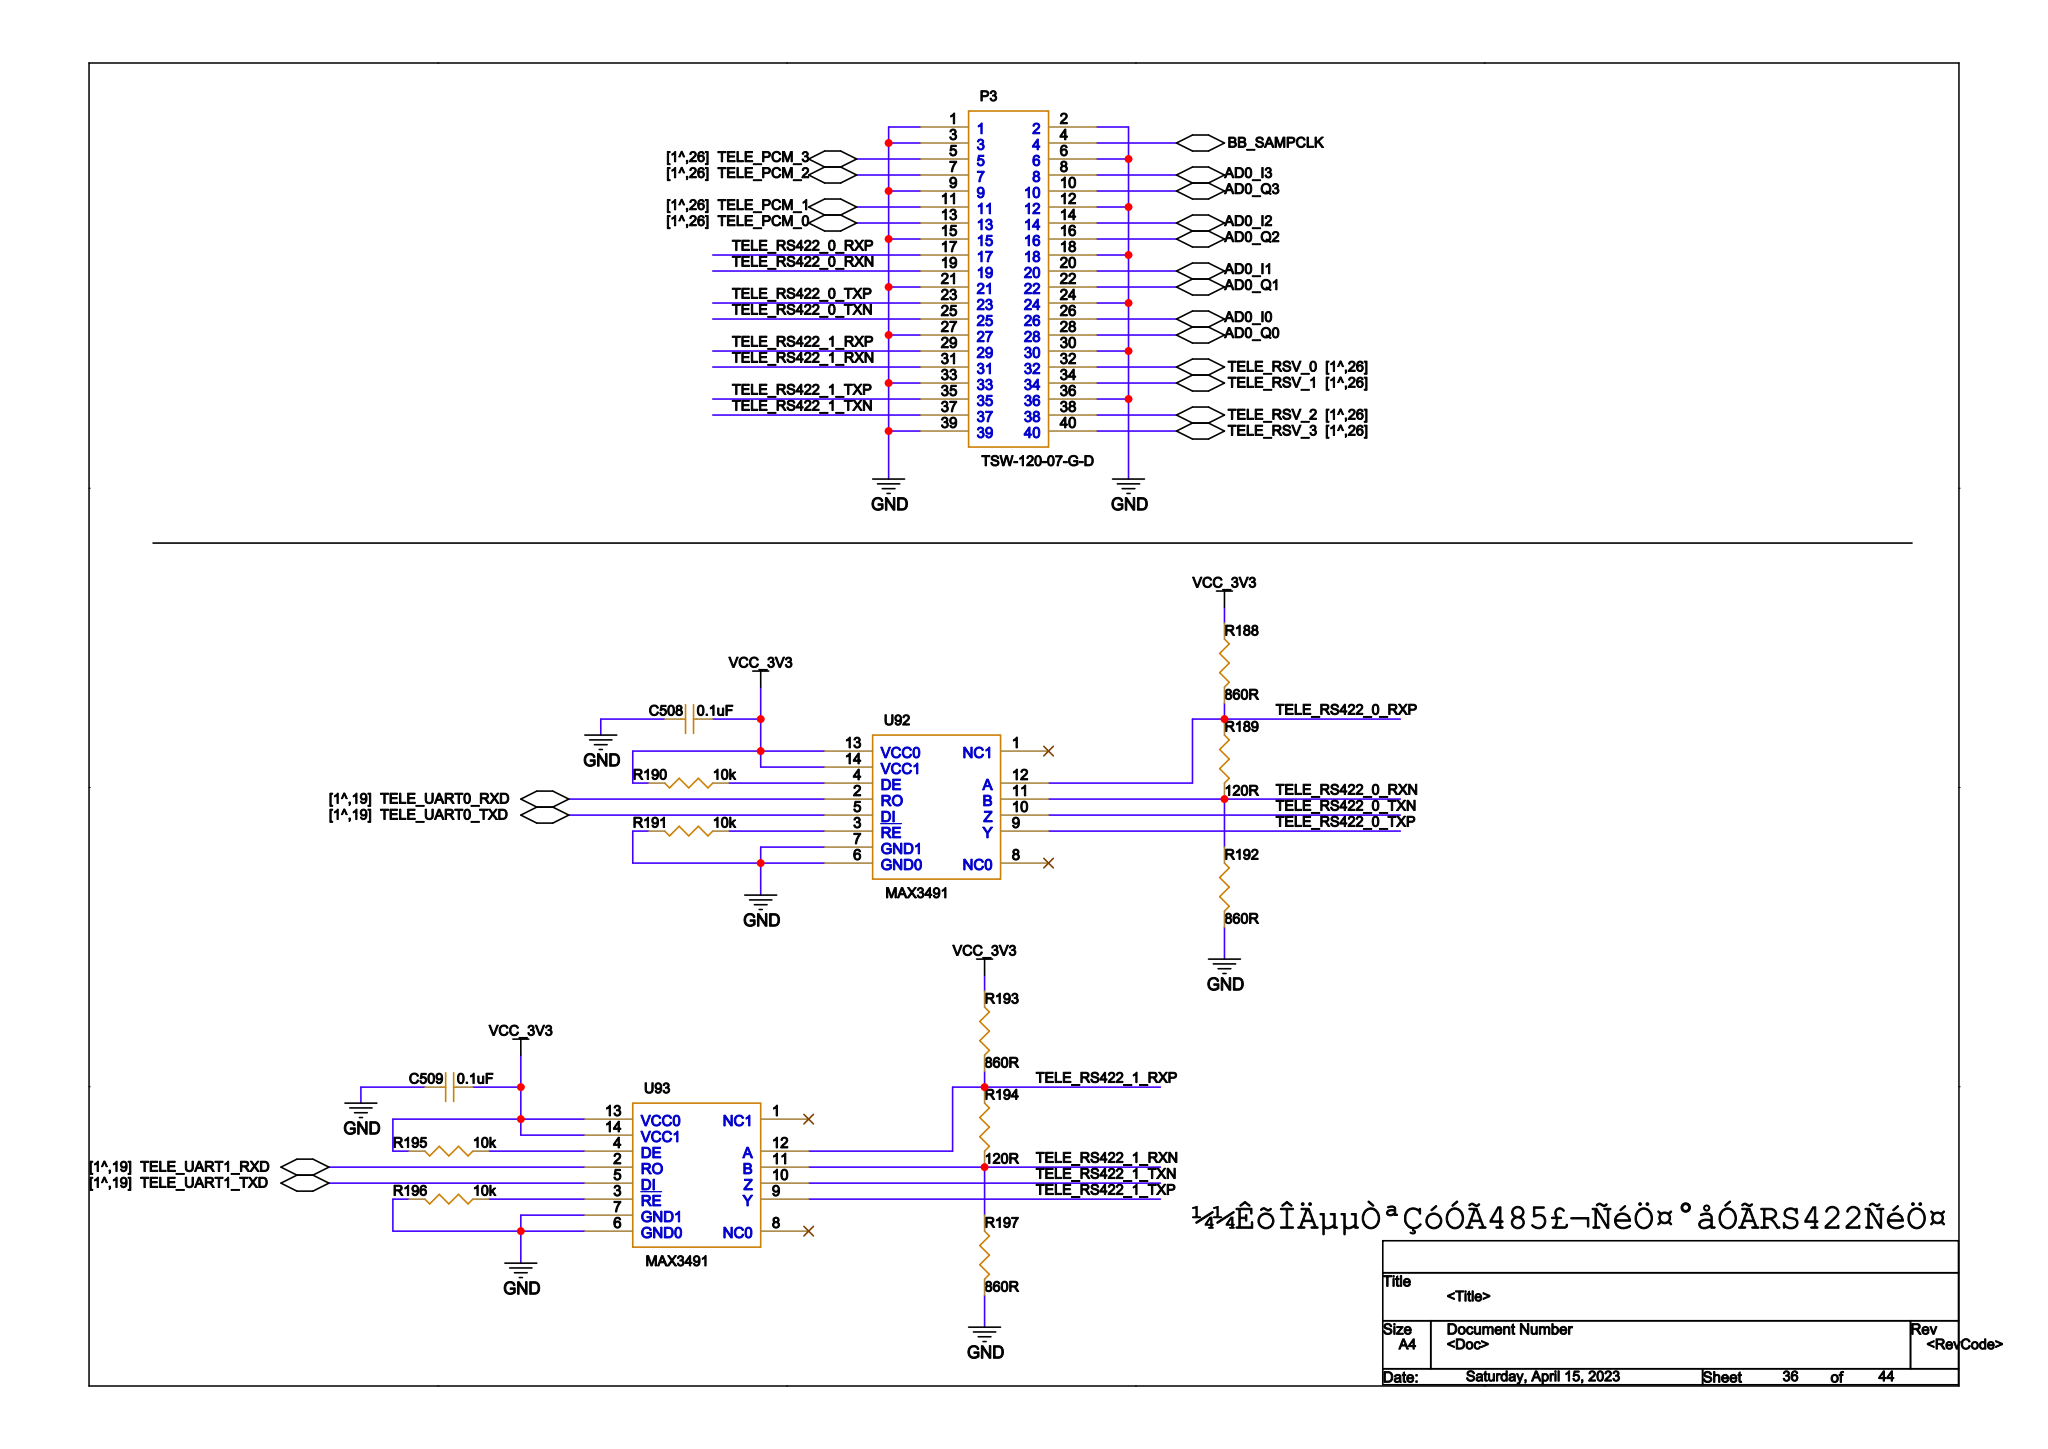Circuit board | Cadence Allegro | 1034 parts | 912 nets | one sheet of the schematic
Parts on this sheet (reference | value | footprint):
C508 | 0.1uF | C0402
C509 | 0.1uF | C0402
P3 | TSW-120-07-G-D | TSW_2MM54_DR
R188 | 860R | R0402
R189 | 120R | R0402
R190 | 10k | R0402
R191 | 10k | R0402
R192 | 860R | R0402
R193 | 860R | R0402
R194 | 120R | R0402
R195 | 10k | R0402
R196 | 10k | R0402
R197 | 860R | R0402
U92 | MAX3491 | MAX3491_14SO
U93 | MAX3491 | MAX3491_14SO
Nets of these parts (net: part-pin ...):
GND: C508-2 C509-2 R191-2 R192-2 R196-2 R197-2 U92-6 U92-7 U93-6 U93-7 P3-1 P3-2 P3-3 P3-6 P3-9 P3-12 P3-15 P3-18 P3-21 P3-24 P3-27 P3-30 P3-33 P3-36 P3-39
VCC_3V3: C508-1 C509-1 R188-1 R190-2 R193-1 R195-2 U92-13 U92-14 U93-13 U93-14
TELE_RS422_0_RXP: R188-2 R189-1 U92-12 P3-17
TELE_RS422_0_RXN: R189-2 R192-1 U92-11 P3-19
TELE_RS422_1_RXP: R193-2 R194-1 U93-12 P3-29
TELE_RS422_1_RXN: R194-2 R197-1 U93-11 P3-31
N13759972: R190-1 U92-4
N234875: U92-5
N234873: U92-2
N13759941: R191-1 U92-3
TELE_RS422_0_TXP: U92-9 P3-23
TELE_RS422_0_TXN: U92-10 P3-25
N13761402: R195-1 U93-4
N234879: U93-5
N234877: U93-2
N13761504: R196-1 U93-3
TELE_RS422_1_TXP: U93-9 P3-35
TELE_RS422_1_TXN: U93-10 P3-37